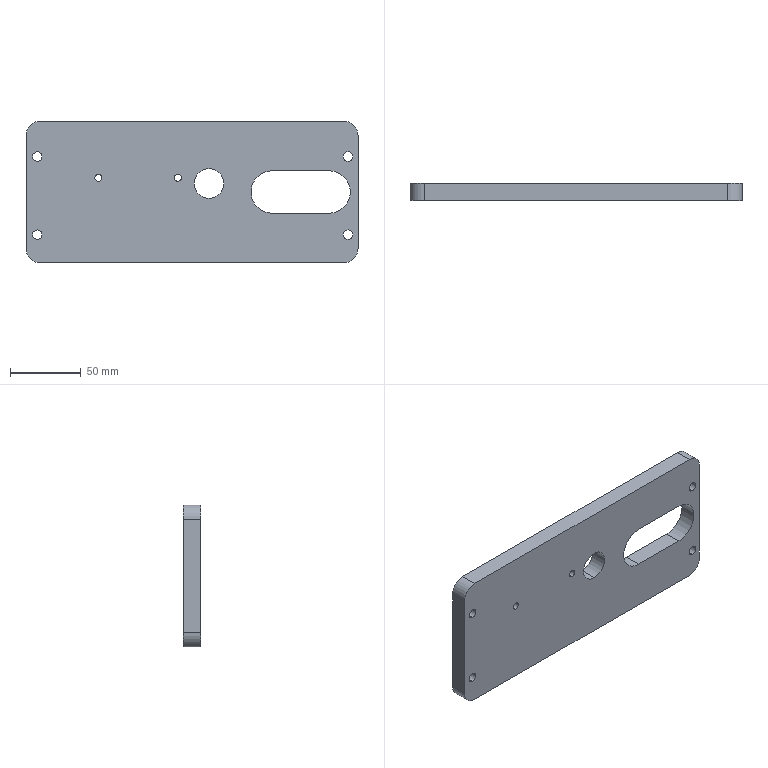Part | STEP file | support plate 6_SUS304 | 1 solid | 56 faces | box 234 x 12 x 100 mm | volume 248248 mm3 | cylinder 36 | plane 12 | cone 8 | commonest cylinder face diameters 4.2 x8 6.6 x8 11 x8 5 x4 20 x4 21 x2